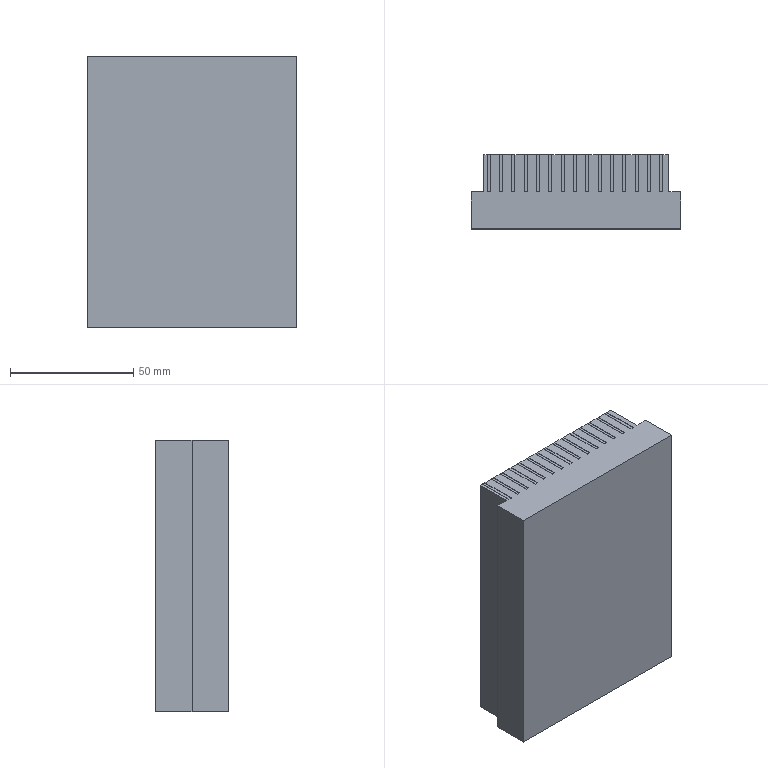Part | SolidWorks | features ICE 2, Extrusion 1, LPattern 1, MirrorPattern 1 | 1 solid | 138 faces | box 85 x 30 x 110 mm | volume 263886 mm3 | plane 138